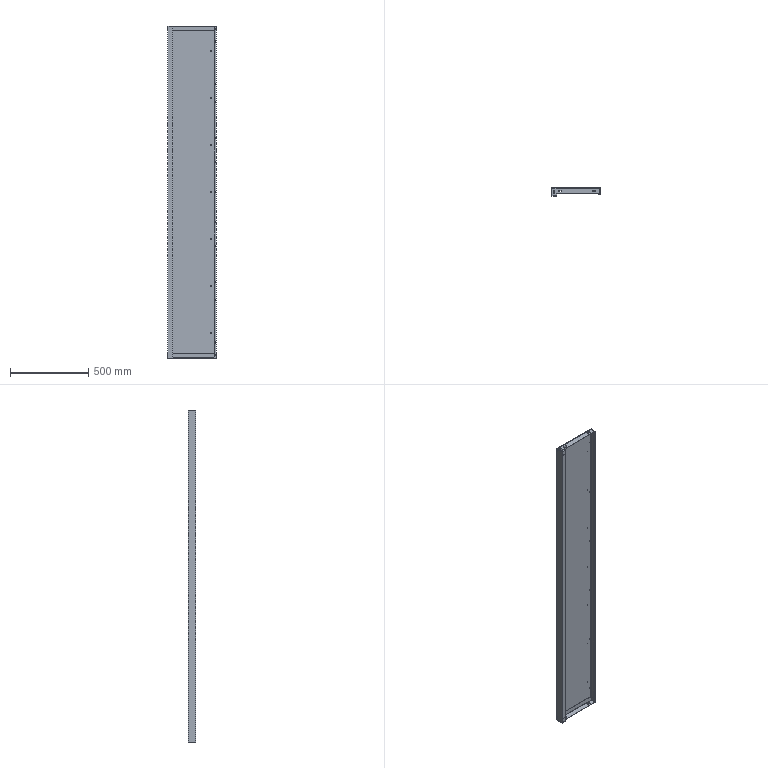Part | SolidWorks | features MirrorCompFeat 1, ReferencePattern 1 | 3 solids | 222 faces | box 310.5 x 50 x 2116 mm | volume 1201289 mm3 | plane 118 | cylinder 104 | commonest cylinder face diameters 6.2 x28 10 x16 4.2 x14 8 x12 11 x12 1 x11